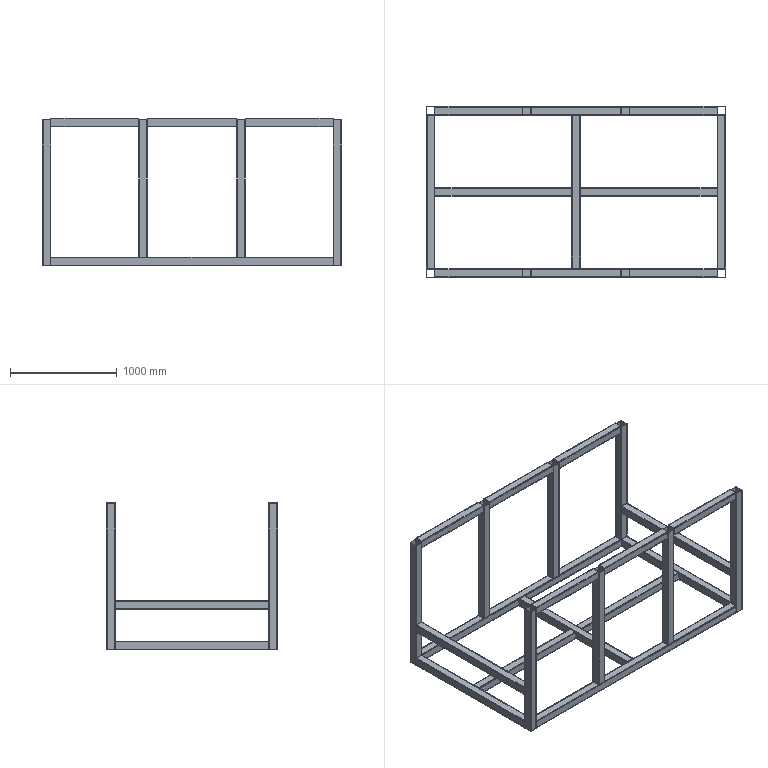Part | STEP file | Part7_default<as machined> | 23 solids | 414 faces | box 2800 x 1600 x 1380 mm | volume 29274094 mm3 | plane 230 | cylinder 184 | commonest cylinder face diameters 6.4 x92 12.8 x92